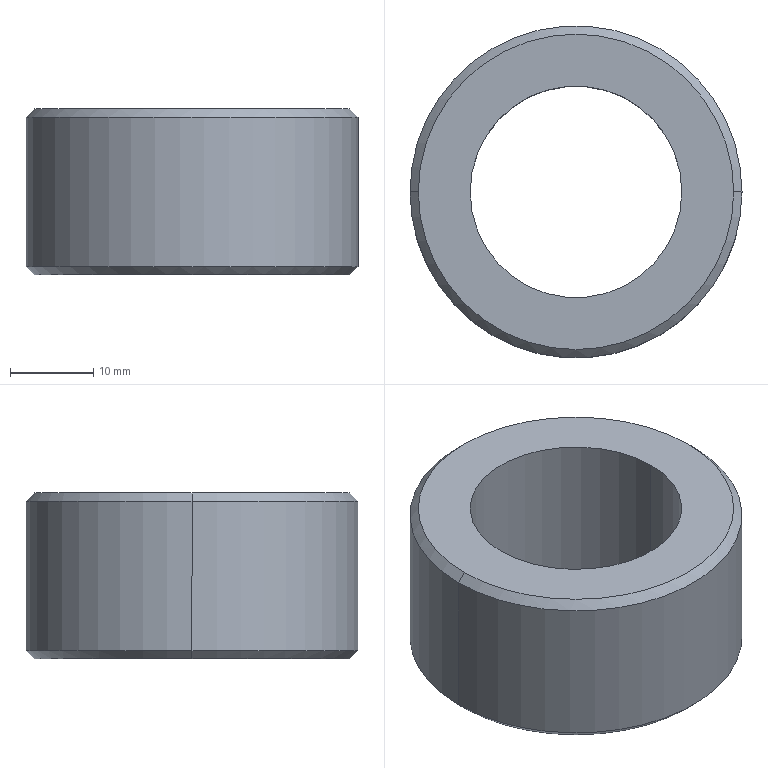Part | STEP file | fBY02F02M-00-19A | 1 solid | 10 faces | box 40 x 40 x 20 mm | volume 14795 mm3 | cylinder 4 | cone 4 | plane 2 | commonest cylinder face diameters 25.5 x2 40 x2
STEP:
#1=CARTESIAN_POINT('',(0.,0.,0.));
#2=DIRECTION('',(0.,0.,1.));
#3=DIRECTION('',(1.,0.,0.));
#4=AXIS2_PLACEMENT_3D('',#1,#2,#3);
#5=CARTESIAN_POINT('',(-20.,0.,19.));
#6=VERTEX_POINT('',#5);
#7=CARTESIAN_POINT('',(20.,0.,19.));
#8=VERTEX_POINT('',#7);
#9=CARTESIAN_POINT('',(0.,0.,19.));
#10=DIRECTION('',(0.,0.,-1.));
#11=DIRECTION('',(-1.,0.,0.));
#12=AXIS2_PLACEMENT_3D('',#9,#10,#11);
#13=CIRCLE('',#12,20.);
#14=CARTESIAN_POINT('',(0.,0.,20.));
#15=DIRECTION('',(0.,0.,-1.));
#16=DIRECTION('',(-1.,0.,0.));
#17=AXIS2_PLACEMENT_3D('',#14,#15,#16);
#18=CYLINDRICAL_SURFACE('',#17,20.);
#19=CARTESIAN_POINT('',(0.,1.));
#20=DIRECTION('',(1.,0.));
#21=VECTOR('',#20,1.);
#22=LINE('',#19,#21);
#23=(GEOMETRIC_REPRESENTATION_CONTEXT(2)PARAMETRIC_REPRESENTATION_CONTEXT()REPRESENTATION_CONTEXT('',''));
#24=DEFINITIONAL_REPRESENTATION('',(#22),#23);
#25=PCURVE('',#18,#24);
#26=CARTESIAN_POINT('',(0.,0.,19.));
#27=DIRECTION('',(0.,0.,-1.));
#28=DIRECTION('',(-1.,0.,0.));
#29=AXIS2_PLACEMENT_3D('',#26,#27,#28);
#30=CONICAL_SURFACE('',#29,20.,0.7854);
#31=CARTESIAN_POINT('',(0.,0.));
#32=DIRECTION('',(1.,0.));
#33=VECTOR('',#32,1.);
#34=LINE('',#31,#33);
#35=(GEOMETRIC_REPRESENTATION_CONTEXT(2)PARAMETRIC_REPRESENTATION_CONTEXT()REPRESENTATION_CONTEXT('',''));
#36=DEFINITIONAL_REPRESENTATION('',(#34),#35);
#37=PCURVE('',#30,#36);
#38=SURFACE_CURVE('',#13,(#25,#37),.PCURVE_S1.);
#39=EDGE_CURVE('',#6,#8,#38,.T.);
#40=ORIENTED_EDGE('',*,*,#39,.T.);
#41=CARTESIAN_POINT('',(20.,0.,1.));
#42=VERTEX_POINT('',#41);
#43=CARTESIAN_POINT('',(20.,0.,20.));
#44=DIRECTION('',(0.,0.,-1.));
#45=VECTOR('',#44,1.);
#46=LINE('',#43,#45);
#47=CARTESIAN_POINT('',(3.142,0.));
#48=DIRECTION('',(0.,1.));
#49=VECTOR('',#48,1.);
#50=LINE('',#47,#49);
#51=(GEOMETRIC_REPRESENTATION_CONTEXT(2)PARAMETRIC_REPRESENTATION_CONTEXT()REPRESENTATION_CONTEXT('',''));
#52=DEFINITIONAL_REPRESENTATION('',(#50),#51);
#53=PCURVE('',#18,#52);
#54=CARTESIAN_POINT('',(0.,0.,20.));
#55=DIRECTION('',(0.,0.,-1.));
#56=DIRECTION('',(-1.,0.,0.));
#57=AXIS2_PLACEMENT_3D('',#54,#55,#56);
#58=CYLINDRICAL_SURFACE('',#57,20.);
#59=CARTESIAN_POINT('',(3.142,0.));
#60=DIRECTION('',(0.,1.));
#61=VECTOR('',#60,1.);
#62=LINE('',#59,#61);
#63=(GEOMETRIC_REPRESENTATION_CONTEXT(2)PARAMETRIC_REPRESENTATION_CONTEXT()REPRESENTATION_CONTEXT('',''));
#64=DEFINITIONAL_REPRESENTATION('',(#62),#63);
#65=PCURVE('',#58,#64);
#66=SURFACE_CURVE('',#46,(#53,#65),.PCURVE_S1.);
#67=EDGE_CURVE('',#8,#42,#66,.T.);
#68=ORIENTED_EDGE('',*,*,#67,.T.);
#69=CARTESIAN_POINT('',(-20.,0.,1.));
#70=VERTEX_POINT('',#69);
#71=CARTESIAN_POINT('',(0.,0.,1.));
#72=DIRECTION('',(0.,0.,1.));
#73=DIRECTION('',(-1.,0.,0.));
#74=AXIS2_PLACEMENT_3D('',#71,#72,#73);
#75=CIRCLE('',#74,20.);
#76=CARTESIAN_POINT('',(6.283,19.));
#77=DIRECTION('',(-1.,0.));
#78=VECTOR('',#77,1.);
#79=LINE('',#76,#78);
#80=(GEOMETRIC_REPRESENTATION_CONTEXT(2)PARAMETRIC_REPRESENTATION_CONTEXT()REPRESENTATION_CONTEXT('',''));
#81=DEFINITIONAL_REPRESENTATION('',(#79),#80);
#82=PCURVE('',#18,#81);
#83=CARTESIAN_POINT('',(0.,0.,1.));
#84=DIRECTION('',(0.,0.,1.));
#85=DIRECTION('',(1.,0.,0.));
#86=AXIS2_PLACEMENT_3D('',#83,#84,#85);
#87=CONICAL_SURFACE('',#86,20.,0.7854);
#88=CARTESIAN_POINT('',(-3.142,0.));
#89=DIRECTION('',(1.,0.));
#90=VECTOR('',#89,1.);
#91=LINE('',#88,#90);
#92=(GEOMETRIC_REPRESENTATION_CONTEXT(2)PARAMETRIC_REPRESENTATION_CONTEXT()REPRESENTATION_CONTEXT('',''));
#93=DEFINITIONAL_REPRESENTATION('',(#91),#92);
#94=PCURVE('',#87,#93);
#95=SURFACE_CURVE('',#75,(#82,#94),.PCURVE_S1.);
#96=EDGE_CURVE('',#42,#70,#95,.T.);
#97=ORIENTED_EDGE('',*,*,#96,.T.);
#98=CARTESIAN_POINT('',(-20.,0.,20.));
#99=DIRECTION('',(0.,0.,-1.));
#100=VECTOR('',#99,1.);
#101=LINE('',#98,#100);
#102=CARTESIAN_POINT('',(0.,0.));
#103=DIRECTION('',(0.,1.));
#104=VECTOR('',#103,1.);
#105=LINE('',#102,#104);
#106=(GEOMETRIC_REPRESENTATION_CONTEXT(2)PARAMETRIC_REPRESENTATION_CONTEXT()REPRESENTATION_CONTEXT('',''));
#107=DEFINITIONAL_REPRESENTATION('',(#105),#106);
#108=PCURVE('',#18,#107);
#109=CARTESIAN_POINT('',(6.283,0.));
#110=DIRECTION('',(0.,1.));
#111=VECTOR('',#110,1.);
#112=LINE('',#109,#111);
#113=(GEOMETRIC_REPRESENTATION_CONTEXT(2)PARAMETRIC_REPRESENTATION_CONTEXT()REPRESENTATION_CONTEXT('',''));
#114=DEFINITIONAL_REPRESENTATION('',(#112),#113);
#115=PCURVE('',#58,#114);
#116=SURFACE_CURVE('',#101,(#108,#115),.PCURVE_S1.);
#117=EDGE_CURVE('',#6,#70,#116,.T.);
#118=ORIENTED_EDGE('',*,*,#117,.F.);
#119=EDGE_LOOP('',(#40,#68,#97,#118));
#120=FACE_BOUND('',#119,.T.);
#121=ADVANCED_FACE('',(#120),#18,.T.);
#122=CARTESIAN_POINT('',(19.,0.,0.));
#123=VERTEX_POINT('',#122);
#124=CARTESIAN_POINT('',(-19.,0.,0.));
#125=VERTEX_POINT('',#124);
#126=CARTESIAN_POINT('',(0.,0.,0.));
#127=DIRECTION('',(0.,0.,1.));
#128=DIRECTION('',(1.,0.,0.));
#129=AXIS2_PLACEMENT_3D('',#126,#127,#128);
#130=CIRCLE('',#129,19.);
#131=CARTESIAN_POINT('',(0.,-1.));
#132=DIRECTION('',(1.,0.));
#133=VECTOR('',#132,1.);
#134=LINE('',#131,#133);
#135=(GEOMETRIC_REPRESENTATION_CONTEXT(2)PARAMETRIC_REPRESENTATION_CONTEXT()REPRESENTATION_CONTEXT('',''));
#136=DEFINITIONAL_REPRESENTATION('',(#134),#135);
#137=PCURVE('',#87,#136);
#138=CARTESIAN_POINT('',(0.,0.,0.));
#139=DIRECTION('',(0.,0.,1.));
#140=DIRECTION('',(1.,0.,0.));
#141=AXIS2_PLACEMENT_3D('',#138,#139,#140);
#142=PLANE('',#141);
#143=CARTESIAN_POINT('',(0.,0.));
#144=DIRECTION('',(1.,0.));
#145=AXIS2_PLACEMENT_2D('',#143,#144);
#146=CIRCLE('',#145,19.);
#147=(GEOMETRIC_REPRESENTATION_CONTEXT(2)PARAMETRIC_REPRESENTATION_CONTEXT()REPRESENTATION_CONTEXT('',''));
#148=DEFINITIONAL_REPRESENTATION('',(#146),#147);
#149=PCURVE('',#142,#148);
#150=SURFACE_CURVE('',#130,(#137,#149),.PCURVE_S1.);
#151=EDGE_CURVE('',#123,#125,#150,.T.);
#152=ORIENTED_EDGE('',*,*,#151,.T.);
#153=CARTESIAN_POINT('',(-20.,0.,1.));
#154=DIRECTION('',(-0.7071,0.,0.7071));
#155=VECTOR('',#154,1.);
#156=LINE('',#153,#155);
#157=CARTESIAN_POINT('',(3.142,0.));
#158=DIRECTION('',(0.,1.));
#159=VECTOR('',#158,1.);
#160=LINE('',#157,#159);
#161=(GEOMETRIC_REPRESENTATION_CONTEXT(2)PARAMETRIC_REPRESENTATION_CONTEXT()REPRESENTATION_CONTEXT('',''));
#162=DEFINITIONAL_REPRESENTATION('',(#160),#161);
#163=PCURVE('',#87,#162);
#164=CARTESIAN_POINT('',(0.,0.,1.));
#165=DIRECTION('',(0.,0.,1.));
#166=DIRECTION('',(1.,0.,0.));
#167=AXIS2_PLACEMENT_3D('',#164,#165,#166);
#168=CONICAL_SURFACE('',#167,20.,0.7854);
#169=CARTESIAN_POINT('',(3.142,0.));
#170=DIRECTION('',(0.,1.));
#171=VECTOR('',#170,1.);
#172=LINE('',#169,#171);
#173=(GEOMETRIC_REPRESENTATION_CONTEXT(2)PARAMETRIC_REPRESENTATION_CONTEXT()REPRESENTATION_CONTEXT('',''));
#174=DEFINITIONAL_REPRESENTATION('',(#172),#173);
#175=PCURVE('',#168,#174);
#176=SURFACE_CURVE('',#156,(#163,#175),.PCURVE_S1.);
#177=EDGE_CURVE('',#125,#70,#176,.T.);
#178=ORIENTED_EDGE('',*,*,#177,.T.);
#179=ORIENTED_EDGE('',*,*,#96,.F.);
#180=CARTESIAN_POINT('',(20.,0.,1.));
#181=DIRECTION('',(0.7071,0.,0.7071));
#182=VECTOR('',#181,1.);
#183=LINE('',#180,#182);
#184=CARTESIAN_POINT('',(0.,0.));
#185=DIRECTION('',(0.,1.));
#186=VECTOR('',#185,1.);
#187=LINE('',#184,#186);
#188=(GEOMETRIC_REPRESENTATION_CONTEXT(2)PARAMETRIC_REPRESENTATION_CONTEXT()REPRESENTATION_CONTEXT('',''));
#189=DEFINITIONAL_REPRESENTATION('',(#187),#188);
#190=PCURVE('',#87,#189);
#191=CARTESIAN_POINT('',(6.283,0.));
#192=DIRECTION('',(0.,1.));
#193=VECTOR('',#192,1.);
#194=LINE('',#191,#193);
#195=(GEOMETRIC_REPRESENTATION_CONTEXT(2)PARAMETRIC_REPRESENTATION_CONTEXT()REPRESENTATION_CONTEXT('',''));
#196=DEFINITIONAL_REPRESENTATION('',(#194),#195);
#197=PCURVE('',#168,#196);
#198=SURFACE_CURVE('',#183,(#190,#197),.PCURVE_S1.);
#199=EDGE_CURVE('',#123,#42,#198,.T.);
#200=ORIENTED_EDGE('',*,*,#199,.F.);
#201=EDGE_LOOP('',(#152,#178,#179,#200));
#202=FACE_BOUND('',#201,.T.);
#203=ADVANCED_FACE('',(#202),#87,.T.);
#204=CARTESIAN_POINT('',(-19.,0.,20.));
#205=VERTEX_POINT('',#204);
#206=CARTESIAN_POINT('',(19.,0.,20.));
#207=VERTEX_POINT('',#206);
#208=CARTESIAN_POINT('',(0.,0.,20.));
#209=DIRECTION('',(0.,0.,-1.));
#210=DIRECTION('',(-1.,0.,0.));
#211=AXIS2_PLACEMENT_3D('',#208,#209,#210);
#212=CIRCLE('',#211,19.);
#213=CARTESIAN_POINT('',(0.,-1.));
#214=DIRECTION('',(1.,0.));
#215=VECTOR('',#214,1.);
#216=LINE('',#213,#215);
#217=(GEOMETRIC_REPRESENTATION_CONTEXT(2)PARAMETRIC_REPRESENTATION_CONTEXT()REPRESENTATION_CONTEXT('',''));
#218=DEFINITIONAL_REPRESENTATION('',(#216),#217);
#219=PCURVE('',#30,#218);
#220=CARTESIAN_POINT('',(0.,0.,20.));
#221=DIRECTION('',(0.,0.,1.));
#222=DIRECTION('',(1.,0.,0.));
#223=AXIS2_PLACEMENT_3D('',#220,#221,#222);
#224=PLANE('',#223);
#225=CARTESIAN_POINT('',(-19.,0.));
#226=CARTESIAN_POINT('',(-19.,32.909));
#227=CARTESIAN_POINT('',(9.5,16.454));
#228=CARTESIAN_POINT('',(38.,0.));
#229=CARTESIAN_POINT('',(9.5,-16.454));
#230=CARTESIAN_POINT('',(-19.,-32.909));
#231=CARTESIAN_POINT('',(-19.,0.));
#232=(BOUNDED_CURVE()B_SPLINE_CURVE(2,(#225,#226,#227,#228,#229,#230,#231),.UNSPECIFIED.,.T.,.F.)B_SPLINE_CURVE_WITH_KNOTS((1,2,2,2,2,1),(-2.094,0.,2.094,4.189,6.283,8.378),.UNSPECIFIED.)CURVE()GEOMETRIC_REPRESENTATION_ITEM()RATIONAL_B_SPLINE_CURVE((1.,0.5,1.,0.5,1.,0.5,1.))REPRESENTATION_ITEM(''));
#233=(GEOMETRIC_REPRESENTATION_CONTEXT(2)PARAMETRIC_REPRESENTATION_CONTEXT()REPRESENTATION_CONTEXT('',''));
#234=DEFINITIONAL_REPRESENTATION('',(#232),#233);
#235=PCURVE('',#224,#234);
#236=SURFACE_CURVE('',#212,(#219,#235),.PCURVE_S1.);
#237=EDGE_CURVE('',#205,#207,#236,.T.);
#238=ORIENTED_EDGE('',*,*,#237,.T.);
#239=CARTESIAN_POINT('',(20.,0.,19.));
#240=DIRECTION('',(0.7071,0.,-0.7071));
#241=VECTOR('',#240,1.);
#242=LINE('',#239,#241);
#243=CARTESIAN_POINT('',(3.142,0.));
#244=DIRECTION('',(0.,1.));
#245=VECTOR('',#244,1.);
#246=LINE('',#243,#245);
#247=(GEOMETRIC_REPRESENTATION_CONTEXT(2)PARAMETRIC_REPRESENTATION_CONTEXT()REPRESENTATION_CONTEXT('',''));
#248=DEFINITIONAL_REPRESENTATION('',(#246),#247);
#249=PCURVE('',#30,#248);
#250=CARTESIAN_POINT('',(0.,0.,19.));
#251=DIRECTION('',(0.,0.,-1.));
#252=DIRECTION('',(-1.,0.,0.));
#253=AXIS2_PLACEMENT_3D('',#250,#251,#252);
#254=CONICAL_SURFACE('',#253,20.,0.7854);
#255=CARTESIAN_POINT('',(3.142,0.));
#256=DIRECTION('',(0.,1.));
#257=VECTOR('',#256,1.);
#258=LINE('',#255,#257);
#259=(GEOMETRIC_REPRESENTATION_CONTEXT(2)PARAMETRIC_REPRESENTATION_CONTEXT()REPRESENTATION_CONTEXT('',''));
#260=DEFINITIONAL_REPRESENTATION('',(#258),#259);
#261=PCURVE('',#254,#260);
#262=SURFACE_CURVE('',#242,(#249,#261),.PCURVE_S1.);
#263=EDGE_CURVE('',#207,#8,#262,.T.);
#264=ORIENTED_EDGE('',*,*,#263,.T.);
#265=ORIENTED_EDGE('',*,*,#39,.F.);
#266=CARTESIAN_POINT('',(-20.,0.,19.));
#267=DIRECTION('',(-0.7071,0.,-0.7071));
#268=VECTOR('',#267,1.);
#269=LINE('',#266,#268);
#270=CARTESIAN_POINT('',(0.,0.));
#271=DIRECTION('',(0.,1.));
#272=VECTOR('',#271,1.);
#273=LINE('',#270,#272);
#274=(GEOMETRIC_REPRESENTATION_CONTEXT(2)PARAMETRIC_REPRESENTATION_CONTEXT()REPRESENTATION_CONTEXT('',''));
#275=DEFINITIONAL_REPRESENTATION('',(#273),#274);
#276=PCURVE('',#30,#275);
#277=CARTESIAN_POINT('',(6.283,0.));
#278=DIRECTION('',(0.,1.));
#279=VECTOR('',#278,1.);
#280=LINE('',#277,#279);
#281=(GEOMETRIC_REPRESENTATION_CONTEXT(2)PARAMETRIC_REPRESENTATION_CONTEXT()REPRESENTATION_CONTEXT('',''));
#282=DEFINITIONAL_REPRESENTATION('',(#280),#281);
#283=PCURVE('',#254,#282);
#284=SURFACE_CURVE('',#269,(#276,#283),.PCURVE_S1.);
#285=EDGE_CURVE('',#205,#6,#284,.T.);
#286=ORIENTED_EDGE('',*,*,#285,.F.);
#287=EDGE_LOOP('',(#238,#264,#265,#286));
#288=FACE_BOUND('',#287,.T.);
#289=ADVANCED_FACE('',(#288),#30,.T.);
#290=CARTESIAN_POINT('',(-12.75,0.,20.));
#291=VERTEX_POINT('',#290);
#292=CARTESIAN_POINT('',(-12.75,0.,0.));
#293=VERTEX_POINT('',#292);
#294=CARTESIAN_POINT('',(-12.75,0.,20.));
#295=DIRECTION('',(0.,0.,-1.));
#296=VECTOR('',#295,1.);
#297=LINE('',#294,#296);
#298=CARTESIAN_POINT('',(0.,0.,20.));
#299=DIRECTION('',(0.,0.,-1.));
#300=DIRECTION('',(-1.,0.,0.));
#301=AXIS2_PLACEMENT_3D('',#298,#299,#300);
#302=CYLINDRICAL_SURFACE('',#301,12.75);
#303=CARTESIAN_POINT('',(6.283,0.));
#304=DIRECTION('',(0.,1.));
#305=VECTOR('',#304,1.);
#306=LINE('',#303,#305);
#307=(GEOMETRIC_REPRESENTATION_CONTEXT(2)PARAMETRIC_REPRESENTATION_CONTEXT()REPRESENTATION_CONTEXT('',''));
#308=DEFINITIONAL_REPRESENTATION('',(#306),#307);
#309=PCURVE('',#302,#308);
#310=CARTESIAN_POINT('',(0.,0.,20.));
#311=DIRECTION('',(0.,0.,-1.));
#312=DIRECTION('',(-1.,0.,0.));
#313=AXIS2_PLACEMENT_3D('',#310,#311,#312);
#314=CYLINDRICAL_SURFACE('',#313,12.75);
#315=CARTESIAN_POINT('',(0.,0.));
#316=DIRECTION('',(0.,1.));
#317=VECTOR('',#316,1.);
#318=LINE('',#315,#317);
#319=(GEOMETRIC_REPRESENTATION_CONTEXT(2)PARAMETRIC_REPRESENTATION_CONTEXT()REPRESENTATION_CONTEXT('',''));
#320=DEFINITIONAL_REPRESENTATION('',(#318),#319);
#321=PCURVE('',#314,#320);
#322=SURFACE_CURVE('',#297,(#309,#321),.PCURVE_S1.);
#323=EDGE_CURVE('',#291,#293,#322,.T.);
#324=ORIENTED_EDGE('',*,*,#323,.T.);
#325=CARTESIAN_POINT('',(12.75,0.,0.));
#326=VERTEX_POINT('',#325);
#327=CARTESIAN_POINT('',(0.,0.,0.));
#328=DIRECTION('',(0.,0.,-1.));
#329=DIRECTION('',(-1.,0.,0.));
#330=AXIS2_PLACEMENT_3D('',#327,#328,#329);
#331=CIRCLE('',#330,12.75);
#332=CARTESIAN_POINT('',(0.,20.));
#333=DIRECTION('',(1.,0.));
#334=VECTOR('',#333,1.);
#335=LINE('',#332,#334);
#336=(GEOMETRIC_REPRESENTATION_CONTEXT(2)PARAMETRIC_REPRESENTATION_CONTEXT()REPRESENTATION_CONTEXT('',''));
#337=DEFINITIONAL_REPRESENTATION('',(#335),#336);
#338=PCURVE('',#302,#337);
#339=CARTESIAN_POINT('',(-12.75,0.));
#340=CARTESIAN_POINT('',(-12.75,22.084));
#341=CARTESIAN_POINT('',(6.375,11.042));
#342=CARTESIAN_POINT('',(25.5,0.));
#343=CARTESIAN_POINT('',(6.375,-11.042));
#344=CARTESIAN_POINT('',(-12.75,-22.084));
#345=CARTESIAN_POINT('',(-12.75,0.));
#346=(BOUNDED_CURVE()B_SPLINE_CURVE(2,(#339,#340,#341,#342,#343,#344,#345),.UNSPECIFIED.,.T.,.F.)B_SPLINE_CURVE_WITH_KNOTS((1,2,2,2,2,1),(-2.094,0.,2.094,4.189,6.283,8.378),.UNSPECIFIED.)CURVE()GEOMETRIC_REPRESENTATION_ITEM()RATIONAL_B_SPLINE_CURVE((1.,0.5,1.,0.5,1.,0.5,1.))REPRESENTATION_ITEM(''));
#347=(GEOMETRIC_REPRESENTATION_CONTEXT(2)PARAMETRIC_REPRESENTATION_CONTEXT()REPRESENTATION_CONTEXT('',''));
#348=DEFINITIONAL_REPRESENTATION('',(#346),#347);
#349=PCURVE('',#142,#348);
#350=SURFACE_CURVE('',#331,(#338,#349),.PCURVE_S1.);
#351=EDGE_CURVE('',#326,#293,#350,.T.);
#352=ORIENTED_EDGE('',*,*,#351,.F.);
#353=CARTESIAN_POINT('',(12.75,0.,20.));
#354=VERTEX_POINT('',#353);
#355=CARTESIAN_POINT('',(12.75,0.,20.));
#356=DIRECTION('',(0.,0.,-1.));
#357=VECTOR('',#356,1.);
#358=LINE('',#355,#357);
#359=CARTESIAN_POINT('',(3.142,0.));
#360=DIRECTION('',(0.,1.));
#361=VECTOR('',#360,1.);
#362=LINE('',#359,#361);
#363=(GEOMETRIC_REPRESENTATION_CONTEXT(2)PARAMETRIC_REPRESENTATION_CONTEXT()REPRESENTATION_CONTEXT('',''));
#364=DEFINITIONAL_REPRESENTATION('',(#362),#363);
#365=PCURVE('',#302,#364);
#366=CARTESIAN_POINT('',(3.142,0.));
#367=DIRECTION('',(0.,1.));
#368=VECTOR('',#367,1.);
#369=LINE('',#366,#368);
#370=(GEOMETRIC_REPRESENTATION_CONTEXT(2)PARAMETRIC_REPRESENTATION_CONTEXT()REPRESENTATION_CONTEXT('',''));
#371=DEFINITIONAL_REPRESENTATION('',(#369),#370);
#372=PCURVE('',#314,#371);
#373=SURFACE_CURVE('',#358,(#365,#372),.PCURVE_S1.);
#374=EDGE_CURVE('',#354,#326,#373,.T.);
#375=ORIENTED_EDGE('',*,*,#374,.F.);
#376=CARTESIAN_POINT('',(0.,0.,20.));
#377=DIRECTION('',(0.,0.,-1.));
#378=DIRECTION('',(-1.,0.,0.));
#379=AXIS2_PLACEMENT_3D('',#376,#377,#378);
#380=CIRCLE('',#379,12.75);
#381=CARTESIAN_POINT('',(0.,0.));
#382=DIRECTION('',(1.,0.));
#383=VECTOR('',#382,1.);
#384=LINE('',#381,#383);
#385=(GEOMETRIC_REPRESENTATION_CONTEXT(2)PARAMETRIC_REPRESENTATION_CONTEXT()REPRESENTATION_CONTEXT('',''));
#386=DEFINITIONAL_REPRESENTATION('',(#384),#385);
#387=PCURVE('',#302,#386);
#388=CARTESIAN_POINT('',(-12.75,0.));
#389=CARTESIAN_POINT('',(-12.75,22.084));
#390=CARTESIAN_POINT('',(6.375,11.042));
#391=CARTESIAN_POINT('',(25.5,0.));
#392=CARTESIAN_POINT('',(6.375,-11.042));
#393=CARTESIAN_POINT('',(-12.75,-22.084));
#394=CARTESIAN_POINT('',(-12.75,0.));
#395=(BOUNDED_CURVE()B_SPLINE_CURVE(2,(#388,#389,#390,#391,#392,#393,#394),.UNSPECIFIED.,.T.,.F.)B_SPLINE_CURVE_WITH_KNOTS((1,2,2,2,2,1),(-2.094,0.,2.094,4.189,6.283,8.378),.UNSPECIFIED.)CURVE()GEOMETRIC_REPRESENTATION_ITEM()RATIONAL_B_SPLINE_CURVE((1.,0.5,1.,0.5,1.,0.5,1.))REPRESENTATION_ITEM(''));
#396=(GEOMETRIC_REPRESENTATION_CONTEXT(2)PARAMETRIC_REPRESENTATION_CONTEXT()REPRESENTATION_CONTEXT('',''));
#397=DEFINITIONAL_REPRESENTATION('',(#395),#396);
#398=PCURVE('',#224,#397);
#399=SURFACE_CURVE('',#380,(#387,#398),.PCURVE_S1.);
#400=EDGE_CURVE('',#354,#291,#399,.T.);
#401=ORIENTED_EDGE('',*,*,#400,.T.);
#402=EDGE_LOOP('',(#324,#352,#375,#401));
#403=FACE_BOUND('',#402,.F.);
#404=ADVANCED_FACE('',(#403),#302,.F.);
#405=ORIENTED_EDGE('',*,*,#67,.F.);
#406=CARTESIAN_POINT('',(0.,0.,19.));
#407=DIRECTION('',(0.,0.,-1.));
#408=DIRECTION('',(-1.,0.,0.));
#409=AXIS2_PLACEMENT_3D('',#406,#407,#408);
#410=CIRCLE('',#409,20.);
#411=CARTESIAN_POINT('',(0.,1.));
#412=DIRECTION('',(1.,0.));
#413=VECTOR('',#412,1.);
#414=LINE('',#411,#413);
#415=(GEOMETRIC_REPRESENTATION_CONTEXT(2)PARAMETRIC_REPRESENTATION_CONTEXT()REPRESENTATION_CONTEXT('',''));
#416=DEFINITIONAL_REPRESENTATION('',(#414),#415);
#417=PCURVE('',#58,#416);
#418=CARTESIAN_POINT('',(0.,0.));
#419=DIRECTION('',(1.,0.));
#420=VECTOR('',#419,1.);
#421=LINE('',#418,#420);
#422=(GEOMETRIC_REPRESENTATION_CONTEXT(2)PARAMETRIC_REPRESENTATION_CONTEXT()REPRESENTATION_CONTEXT('',''));
#423=DEFINITIONAL_REPRESENTATION('',(#421),#422);
#424=PCURVE('',#254,#423);
#425=SURFACE_CURVE('',#410,(#417,#424),.PCURVE_S1.);
#426=EDGE_CURVE('',#8,#6,#425,.T.);
#427=ORIENTED_EDGE('',*,*,#426,.T.);
#428=ORIENTED_EDGE('',*,*,#117,.T.);
#429=CARTESIAN_POINT('',(0.,0.,1.));
#430=DIRECTION('',(0.,0.,1.));
#431=DIRECTION('',(-1.,0.,0.));
#432=AXIS2_PLACEMENT_3D('',#429,#430,#431);
#433=CIRCLE('',#432,20.);
#434=CARTESIAN_POINT('',(6.283,19.));
#435=DIRECTION('',(-1.,0.));
#436=VECTOR('',#435,1.);
#437=LINE('',#434,#436);
#438=(GEOMETRIC_REPRESENTATION_CONTEXT(2)PARAMETRIC_REPRESENTATION_CONTEXT()REPRESENTATION_CONTEXT('',''));
#439=DEFINITIONAL_REPRESENTATION('',(#437),#438);
#440=PCURVE('',#58,#439);
#441=CARTESIAN_POINT('',(3.142,0.));
#442=DIRECTION('',(1.,0.));
#443=VECTOR('',#442,1.);
#444=LINE('',#441,#443);
#445=(GEOMETRIC_REPRESENTATION_CONTEXT(2)PARAMETRIC_REPRESENTATION_CONTEXT()REPRESENTATION_CONTEXT('',''));
#446=DEFINITIONAL_REPRESENTATION('',(#444),#445);
#447=PCURVE('',#168,#446);
#448=SURFACE_CURVE('',#433,(#440,#447),.PCURVE_S1.);
#449=EDGE_CURVE('',#70,#42,#448,.T.);
#450=ORIENTED_EDGE('',*,*,#449,.T.);
#451=EDGE_LOOP('',(#405,#427,#428,#450));
#452=FACE_BOUND('',#451,.T.);
#453=ADVANCED_FACE('',(#452),#58,.T.);
#454=ORIENTED_EDGE('',*,*,#177,.F.);
#455=CARTESIAN_POINT('',(0.,0.,0.));
#456=DIRECTION('',(0.,0.,1.));
#457=DIRECTION('',(1.,0.,0.));
#458=AXIS2_PLACEMENT_3D('',#455,#456,#457);
#459=CIRCLE('',#458,19.);
#460=CARTESIAN_POINT('',(0.,-1.));
#461=DIRECTION('',(1.,0.));
#462=VECTOR('',#461,1.);
#463=LINE('',#460,#462);
#464=(GEOMETRIC_REPRESENTATION_CONTEXT(2)PARAMETRIC_REPRESENTATION_CONTEXT()REPRESENTATION_CONTEXT('',''));
#465=DEFINITIONAL_REPRESENTATION('',(#463),#464);
#466=PCURVE('',#168,#465);
#467=CARTESIAN_POINT('',(0.,0.));
#468=DIRECTION('',(1.,0.));
#469=AXIS2_PLACEMENT_2D('',#467,#468);
#470=CIRCLE('',#469,19.);
#471=(GEOMETRIC_REPRESENTATION_CONTEXT(2)PARAMETRIC_REPRESENTATION_CONTEXT()REPRESENTATION_CONTEXT('',''));
#472=DEFINITIONAL_REPRESENTATION('',(#470),#471);
#473=PCURVE('',#142,#472);
#474=SURFACE_CURVE('',#459,(#466,#473),.PCURVE_S1.);
#475=EDGE_CURVE('',#125,#123,#474,.T.);
#476=ORIENTED_EDGE('',*,*,#475,.T.);
#477=ORIENTED_EDGE('',*,*,#199,.T.);
#478=ORIENTED_EDGE('',*,*,#449,.F.);
#479=EDGE_LOOP('',(#454,#476,#477,#478));
#480=FACE_BOUND('',#479,.T.);
#481=ADVANCED_FACE('',(#480),#168,.T.);
#482=ORIENTED_EDGE('',*,*,#263,.F.);
#483=CARTESIAN_POINT('',(0.,0.,20.));
#484=DIRECTION('',(0.,0.,-1.));
#485=DIRECTION('',(-1.,0.,0.));
#486=AXIS2_PLACEMENT_3D('',#483,#484,#485);
#487=CIRCLE('',#486,19.);
#488=CARTESIAN_POINT('',(0.,-1.));
#489=DIRECTION('',(1.,0.));
#490=VECTOR('',#489,1.);
#491=LINE('',#488,#490);
#492=(GEOMETRIC_REPRESENTATION_CONTEXT(2)PARAMETRIC_REPRESENTATION_CONTEXT()REPRESENTATION_CONTEXT('',''));
#493=DEFINITIONAL_REPRESENTATION('',(#491),#492);
#494=PCURVE('',#254,#493);
#495=CARTESIAN_POINT('',(-19.,0.));
#496=CARTESIAN_POINT('',(-19.,32.909));
#497=CARTESIAN_POINT('',(9.5,16.454));
#498=CARTESIAN_POINT('',(38.,0.));
#499=CARTESIAN_POINT('',(9.5,-16.454));
#500=CARTESIAN_POINT('',(-19.,-32.909));
#501=CARTESIAN_POINT('',(-19.,0.));
#502=(BOUNDED_CURVE()B_SPLINE_CURVE(2,(#495,#496,#497,#498,#499,#500,#501),.UNSPECIFIED.,.T.,.F.)B_SPLINE_CURVE_WITH_KNOTS((1,2,2,2,2,1),(-2.094,0.,2.094,4.189,6.283,8.378),.UNSPECIFIED.)CURVE()GEOMETRIC_REPRESENTATION_ITEM()RATIONAL_B_SPLINE_CURVE((1.,0.5,1.,0.5,1.,0.5,1.))REPRESENTATION_ITEM(''));
#503=(GEOMETRIC_REPRESENTATION_CONTEXT(2)PARAMETRIC_REPRESENTATION_CONTEXT()REPRESENTATION_CONTEXT('',''));
#504=DEFINITIONAL_REPRESENTATION('',(#502),#503);
#505=PCURVE('',#224,#504);
#506=SURFACE_CURVE('',#487,(#494,#505),.PCURVE_S1.);
#507=EDGE_CURVE('',#207,#205,#506,.T.);
#508=ORIENTED_EDGE('',*,*,#507,.T.);
#509=ORIENTED_EDGE('',*,*,#285,.T.);
#510=ORIENTED_EDGE('',*,*,#426,.F.);
#511=EDGE_LOOP('',(#482,#508,#509,#510));
#512=FACE_BOUND('',#511,.T.);
#513=ADVANCED_FACE('',(#512),#254,.T.);
#514=CARTESIAN_POINT('',(0.,0.,0.));
#515=DIRECTION('',(0.,0.,-1.));
#516=DIRECTION('',(-1.,0.,0.));
#517=AXIS2_PLACEMENT_3D('',#514,#515,#516);
#518=CIRCLE('',#517,12.75);
#519=CARTESIAN_POINT('',(-12.75,0.));
#520=CARTESIAN_POINT('',(-12.75,22.084));
#521=CARTESIAN_POINT('',(6.375,11.042));
#522=CARTESIAN_POINT('',(25.5,0.));
#523=CARTESIAN_POINT('',(6.375,-11.042));
#524=CARTESIAN_POINT('',(-12.75,-22.084));
#525=CARTESIAN_POINT('',(-12.75,0.));
#526=(BOUNDED_CURVE()B_SPLINE_CURVE(2,(#519,#520,#521,#522,#523,#524,#525),.UNSPECIFIED.,.T.,.F.)B_SPLINE_CURVE_WITH_KNOTS((1,2,2,2,2,1),(-2.094,0.,2.094,4.189,6.283,8.378),.UNSPECIFIED.)CURVE()GEOMETRIC_REPRESENTATION_ITEM()RATIONAL_B_SPLINE_CURVE((1.,0.5,1.,0.5,1.,0.5,1.))REPRESENTATION_ITEM(''));
#527=(GEOMETRIC_REPRESENTATION_CONTEXT(2)PARAMETRIC_REPRESENTATION_CONTEXT()REPRESENTATION_CONTEXT('',''));
#528=DEFINITIONAL_REPRESENTATION('',(#526),#527);
#529=PCURVE('',#142,#528);
#530=CARTESIAN_POINT('',(0.,20.));
#531=DIRECTION('',(1.,0.));
#532=VECTOR('',#531,1.);
#533=LINE('',#530,#532);
#534=(GEOMETRIC_REPRESENTATION_CONTEXT(2)PARAMETRIC_REPRESENTATION_CONTEXT()REPRESENTATION_CONTEXT('',''));
#535=DEFINITIONAL_REPRESENTATION('',(#533),#534);
#536=PCURVE('',#314,#535);
#537=SURFACE_CURVE('',#518,(#529,#536),.PCURVE_S1.);
#538=EDGE_CURVE('',#293,#326,#537,.T.);
#539=ORIENTED_EDGE('',*,*,#538,.F.);
#540=ORIENTED_EDGE('',*,*,#351,.F.);
#541=EDGE_LOOP('',(#539,#540));
#542=FACE_BOUND('',#541,.T.);
#543=ORIENTED_EDGE('',*,*,#151,.F.);
#544=ORIENTED_EDGE('',*,*,#475,.F.);
#545=EDGE_LOOP('',(#543,#544));
#546=FACE_BOUND('',#545,.T.);
#547=ADVANCED_FACE('',(#542,#546),#142,.F.);
#548=CARTESIAN_POINT('',(0.,0.,20.));
#549=DIRECTION('',(0.,0.,-1.));
#550=DIRECTION('',(-1.,0.,0.));
#551=AXIS2_PLACEMENT_3D('',#548,#549,#550);
#552=CIRCLE('',#551,12.75);
#553=CARTESIAN_POINT('',(-12.75,0.));
#554=CARTESIAN_POINT('',(-12.75,22.084));
#555=CARTESIAN_POINT('',(6.375,11.042));
#556=CARTESIAN_POINT('',(25.5,0.));
#557=CARTESIAN_POINT('',(6.375,-11.042));
#558=CARTESIAN_POINT('',(-12.75,-22.084));
#559=CARTESIAN_POINT('',(-12.75,0.));
#560=(BOUNDED_CURVE()B_SPLINE_CURVE(2,(#553,#554,#555,#556,#557,#558,#559),.UNSPECIFIED.,.T.,.F.)B_SPLINE_CURVE_WITH_KNOTS((1,2,2,2,2,1),(-2.094,0.,2.094,4.189,6.283,8.378),.UNSPECIFIED.)CURVE()GEOMETRIC_REPRESENTATION_ITEM()RATIONAL_B_SPLINE_CURVE((1.,0.5,1.,0.5,1.,0.5,1.))REPRESENTATION_ITEM(''));
#561=(GEOMETRIC_REPRESENTATION_CONTEXT(2)PARAMETRIC_REPRESENTATION_CONTEXT()REPRESENTATION_CONTEXT('',''));
#562=DEFINITIONAL_REPRESENTATION('',(#560),#561);
#563=PCURVE('',#224,#562);
#564=CARTESIAN_POINT('',(0.,0.));
#565=DIRECTION('',(1.,0.));
#566=VECTOR('',#565,1.);
#567=LINE('',#564,#566);
#568=(GEOMETRIC_REPRESENTATION_CONTEXT(2)PARAMETRIC_REPRESENTATION_CONTEXT()REPRESENTATION_CONTEXT('',''));
#569=DEFINITIONAL_REPRESENTATION('',(#567),#568);
#570=PCURVE('',#314,#569);
#571=SURFACE_CURVE('',#552,(#563,#570),.PCURVE_S1.);
#572=EDGE_CURVE('',#291,#354,#571,.T.);
#573=ORIENTED_EDGE('',*,*,#572,.T.);
#574=ORIENTED_EDGE('',*,*,#400,.T.);
#575=EDGE_LOOP('',(#573,#574));
#576=FACE_BOUND('',#575,.T.);
#577=ORIENTED_EDGE('',*,*,#237,.F.);
#578=ORIENTED_EDGE('',*,*,#507,.F.);
#579=EDGE_LOOP('',(#577,#578));
#580=FACE_BOUND('',#579,.T.);
#581=ADVANCED_FACE('',(#576,#580),#224,.T.);
#582=ORIENTED_EDGE('',*,*,#538,.F.);
#583=ORIENTED_EDGE('',*,*,#323,.F.);
#584=ORIENTED_EDGE('',*,*,#572,.T.);
#585=ORIENTED_EDGE('',*,*,#374,.T.);
#586=EDGE_LOOP('',(#582,#583,#584,#585));
#587=FACE_BOUND('',#586,.F.);
#588=ADVANCED_FACE('',(#587),#314,.F.);
#589=CLOSED_SHELL('',(#121,#203,#289,#404,#453,#481,#513,#547,#581,#588));
#590=MANIFOLD_SOLID_BREP('',#589);
#591=(LENGTH_UNIT()NAMED_UNIT(*)SI_UNIT(.MILLI.,.METRE.));
#592=UNCERTAINTY_MEASURE_WITH_UNIT(LENGTH_MEASURE(0.0000001),#591,'','');
#593=(NAMED_UNIT(*)PLANE_ANGLE_UNIT()SI_UNIT($,.RADIAN.));
#594=(NAMED_UNIT(*)SI_UNIT($,.STERADIAN.)SOLID_ANGLE_UNIT());
#595=(GEOMETRIC_REPRESENTATION_CONTEXT(3)GLOBAL_UNCERTAINTY_ASSIGNED_CONTEXT((#592))GLOBAL_UNIT_ASSIGNED_CONTEXT((#591,#593,#594))REPRESENTATION_CONTEXT('',''));
#596=ADVANCED_BREP_SHAPE_REPRESENTATION('',(#4,#590),#595);